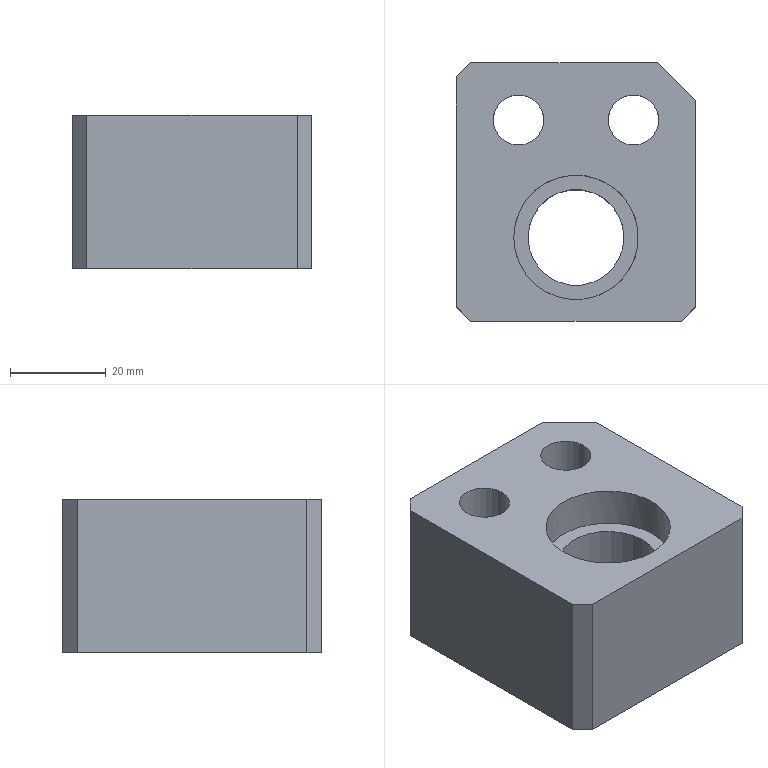Part | STEP file | lll_id3578_x_t | 1 solid | 19 faces | box 50 x 54 x 32 mm | volume 62798 mm3 | plane 13 | cylinder 6 | commonest cylinder face diameters 10.5 x2 17 x2 20 x1 26 x1
STEP:
#1=CARTESIAN_POINT('',(3209.75,-131.,77.5));
#2=VERTEX_POINT('',#1);
#3=CARTESIAN_POINT('',(3215.,-131.,77.5));
#4=DIRECTION('',(0.,0.,1.));
#5=DIRECTION('',(-1.,0.,0.));
#6=AXIS2_PLACEMENT_3D('',#3,#4,#5);
#7=CIRCLE('',#6,5.25);
#8=EDGE_CURVE('',#2,#2,#7,.T.);
#9=ORIENTED_EDGE('',*,*,#8,.T.);
#10=EDGE_LOOP('',(#9));
#11=FACE_BOUND('',#10,.T.);
#12=CARTESIAN_POINT('',(3206.5,-131.,77.5));
#13=VERTEX_POINT('',#12);
#14=CARTESIAN_POINT('',(3215.,-131.,77.5));
#15=DIRECTION('',(0.,0.,1.));
#16=DIRECTION('',(-1.,0.,0.));
#17=AXIS2_PLACEMENT_3D('',#14,#15,#16);
#18=CIRCLE('',#17,8.5);
#19=EDGE_CURVE('',#13,#13,#18,.T.);
#20=ORIENTED_EDGE('',*,*,#19,.F.);
#21=EDGE_LOOP('',(#20));
#22=FACE_BOUND('',#21,.T.);
#23=CARTESIAN_POINT('',(3215.,-131.,77.5));
#24=DIRECTION('',(0.,0.,1.));
#25=DIRECTION('',(-1.,0.,0.));
#26=AXIS2_PLACEMENT_3D('',#23,#24,#25);
#27=PLANE('',#26);
#28=ADVANCED_FACE('',(#11,#22),#27,.F.);
#29=CARTESIAN_POINT('',(3216.,-155.5,84.3));
#30=VERTEX_POINT('',#29);
#31=CARTESIAN_POINT('',(3203.,-155.5,84.3));
#32=DIRECTION('',(0.,0.,1.));
#33=DIRECTION('',(1.,0.,0.));
#34=AXIS2_PLACEMENT_3D('',#31,#32,#33);
#35=CIRCLE('',#34,13.);
#36=EDGE_CURVE('',#30,#30,#35,.T.);
#37=ORIENTED_EDGE('',*,*,#36,.T.);
#38=EDGE_LOOP('',(#37));
#39=FACE_BOUND('',#38,.T.);
#40=CARTESIAN_POINT('',(3193.,-155.5,84.3));
#41=VERTEX_POINT('',#40);
#42=CARTESIAN_POINT('',(3203.,-155.5,84.3));
#43=DIRECTION('',(0.,0.,1.));
#44=DIRECTION('',(-1.,0.,0.));
#45=AXIS2_PLACEMENT_3D('',#42,#43,#44);
#46=CIRCLE('',#45,10.);
#47=EDGE_CURVE('',#41,#41,#46,.T.);
#48=ORIENTED_EDGE('',*,*,#47,.F.);
#49=EDGE_LOOP('',(#48));
#50=FACE_BOUND('',#49,.T.);
#51=CARTESIAN_POINT('',(3203.,-146.75,84.3));
#52=DIRECTION('',(0.,0.,-1.));
#53=DIRECTION('',(0.,1.,0.));
#54=AXIS2_PLACEMENT_3D('',#51,#52,#53);
#55=PLANE('',#54);
#56=ADVANCED_FACE('',(#39,#50),#55,.F.);
#57=ORIENTED_EDGE('',*,*,#19,.T.);
#58=EDGE_LOOP('',(#57));
#59=FACE_BOUND('',#58,.T.);
#60=CARTESIAN_POINT('',(3206.5,-131.,60.5));
#61=VERTEX_POINT('',#60);
#62=CARTESIAN_POINT('',(3215.,-131.,60.5));
#63=DIRECTION('',(0.,0.,-1.));
#64=DIRECTION('',(-1.,0.,0.));
#65=AXIS2_PLACEMENT_3D('',#62,#63,#64);
#66=CIRCLE('',#65,8.5);
#67=EDGE_CURVE('',#61,#61,#66,.T.);
#68=ORIENTED_EDGE('',*,*,#67,.T.);
#69=EDGE_LOOP('',(#68));
#70=FACE_BOUND('',#69,.T.);
#71=CARTESIAN_POINT('',(3215.,-131.,60.5));
#72=DIRECTION('',(0.,0.,1.));
#73=DIRECTION('',(-1.,0.,0.));
#74=AXIS2_PLACEMENT_3D('',#71,#72,#73);
#75=CYLINDRICAL_SURFACE('',#74,8.5);
#76=ADVANCED_FACE('',(#59,#70),#75,.F.);
#77=CARTESIAN_POINT('',(3228.,-127.,60.5));
#78=VERTEX_POINT('',#77);
#79=CARTESIAN_POINT('',(3220.,-119.,60.5));
#80=VERTEX_POINT('',#79);
#81=CARTESIAN_POINT('',(3220.,-119.,60.5));
#82=DIRECTION('',(-0.7071,0.7071,0.));
#83=VECTOR('',#82,1.);
#84=LINE('',#81,#83);
#85=EDGE_CURVE('',#78,#80,#84,.T.);
#86=ORIENTED_EDGE('',*,*,#85,.T.);
#87=CARTESIAN_POINT('',(3220.,-119.,92.5));
#88=VERTEX_POINT('',#87);
#89=CARTESIAN_POINT('',(3220.,-119.,-8.5));
#90=DIRECTION('',(0.,0.,1.));
#91=VECTOR('',#90,1.);
#92=LINE('',#89,#91);
#93=EDGE_CURVE('',#80,#88,#92,.T.);
#94=ORIENTED_EDGE('',*,*,#93,.T.);
#95=CARTESIAN_POINT('',(3228.,-127.,92.5));
#96=VERTEX_POINT('',#95);
#97=CARTESIAN_POINT('',(3220.,-119.,92.5));
#98=DIRECTION('',(0.7071,-0.7071,0.));
#99=VECTOR('',#98,1.);
#100=LINE('',#97,#99);
#101=EDGE_CURVE('',#88,#96,#100,.T.);
#102=ORIENTED_EDGE('',*,*,#101,.T.);
#103=CARTESIAN_POINT('',(3228.,-127.,-8.5));
#104=DIRECTION('',(0.,0.,-1.));
#105=VECTOR('',#104,1.);
#106=LINE('',#103,#105);
#107=EDGE_CURVE('',#96,#78,#106,.T.);
#108=ORIENTED_EDGE('',*,*,#107,.T.);
#109=EDGE_LOOP('',(#86,#94,#102,#108));
#110=FACE_OUTER_BOUND('',#109,.T.);
#111=CARTESIAN_POINT('',(3220.,-119.,-8.5));
#112=DIRECTION('',(-0.7071,-0.7071,0.));
#113=DIRECTION('',(0.7071,-0.7071,0.));
#114=AXIS2_PLACEMENT_3D('',#111,#112,#113);
#115=PLANE('',#114);
#116=ADVANCED_FACE('',(#110),#115,.F.);
#117=CARTESIAN_POINT('',(3228.,-170.,92.5));
#118=VERTEX_POINT('',#117);
#119=CARTESIAN_POINT('',(3228.,-124.275,92.5));
#120=DIRECTION('',(0.,1.,0.));
#121=VECTOR('',#120,1.);
#122=LINE('',#119,#121);
#123=EDGE_CURVE('',#118,#96,#122,.T.);
#124=ORIENTED_EDGE('',*,*,#123,.F.);
#125=CARTESIAN_POINT('',(3228.,-170.,60.5));
#126=VERTEX_POINT('',#125);
#127=CARTESIAN_POINT('',(3228.,-170.,-8.5));
#128=DIRECTION('',(0.,0.,1.));
#129=VECTOR('',#128,1.);
#130=LINE('',#127,#129);
#131=EDGE_CURVE('',#126,#118,#130,.T.);
#132=ORIENTED_EDGE('',*,*,#131,.F.);
#133=CARTESIAN_POINT('',(3228.,-124.275,60.5));
#134=DIRECTION('',(0.,-1.,0.));
#135=VECTOR('',#134,1.);
#136=LINE('',#133,#135);
#137=EDGE_CURVE('',#78,#126,#136,.T.);
#138=ORIENTED_EDGE('',*,*,#137,.F.);
#139=ORIENTED_EDGE('',*,*,#107,.F.);
#140=EDGE_LOOP('',(#124,#132,#138,#139));
#141=FACE_OUTER_BOUND('',#140,.T.);
#142=CARTESIAN_POINT('',(3228.,-155.5,-8.5));
#143=DIRECTION('',(1.,0.,0.));
#144=DIRECTION('',(0.,0.,1.));
#145=AXIS2_PLACEMENT_3D('',#142,#143,#144);
#146=PLANE('',#145);
#147=ADVANCED_FACE('',(#141),#146,.T.);
#148=CARTESIAN_POINT('',(3225.,-173.,92.5));
#149=VERTEX_POINT('',#148);
#150=CARTESIAN_POINT('',(3225.,-173.,92.5));
#151=DIRECTION('',(-0.7071,-0.7071,0.));
#152=VECTOR('',#151,1.);
#153=LINE('',#150,#152);
#154=EDGE_CURVE('',#118,#149,#153,.T.);
#155=ORIENTED_EDGE('',*,*,#154,.T.);
#156=CARTESIAN_POINT('',(3225.,-173.,60.5));
#157=VERTEX_POINT('',#156);
#158=CARTESIAN_POINT('',(3225.,-173.,-8.5));
#159=DIRECTION('',(0.,0.,-1.));
#160=VECTOR('',#159,1.);
#161=LINE('',#158,#160);
#162=EDGE_CURVE('',#149,#157,#161,.T.);
#163=ORIENTED_EDGE('',*,*,#162,.T.);
#164=CARTESIAN_POINT('',(3225.,-173.,60.5));
#165=DIRECTION('',(0.7071,0.7071,0.));
#166=VECTOR('',#165,1.);
#167=LINE('',#164,#166);
#168=EDGE_CURVE('',#157,#126,#167,.T.);
#169=ORIENTED_EDGE('',*,*,#168,.T.);
#170=ORIENTED_EDGE('',*,*,#131,.T.);
#171=EDGE_LOOP('',(#155,#163,#169,#170));
#172=FACE_OUTER_BOUND('',#171,.T.);
#173=CARTESIAN_POINT('',(3225.,-173.,-8.5));
#174=DIRECTION('',(-0.7071,0.7071,0.));
#175=DIRECTION('',(-0.7071,-0.7071,0.));
#176=AXIS2_PLACEMENT_3D('',#173,#174,#175);
#177=PLANE('',#176);
#178=ADVANCED_FACE('',(#172),#177,.F.);
#179=CARTESIAN_POINT('',(3181.,-173.,92.5));
#180=VERTEX_POINT('',#179);
#181=CARTESIAN_POINT('',(3203.,-173.,92.5));
#182=DIRECTION('',(1.,0.,0.));
#183=VECTOR('',#182,1.);
#184=LINE('',#181,#183);
#185=EDGE_CURVE('',#180,#149,#184,.T.);
#186=ORIENTED_EDGE('',*,*,#185,.F.);
#187=CARTESIAN_POINT('',(3181.,-173.,60.5));
#188=VERTEX_POINT('',#187);
#189=CARTESIAN_POINT('',(3181.,-173.,-8.5));
#190=DIRECTION('',(0.,0.,1.));
#191=VECTOR('',#190,1.);
#192=LINE('',#189,#191);
#193=EDGE_CURVE('',#188,#180,#192,.T.);
#194=ORIENTED_EDGE('',*,*,#193,.F.);
#195=CARTESIAN_POINT('',(3203.,-173.,60.5));
#196=DIRECTION('',(-1.,0.,0.));
#197=VECTOR('',#196,1.);
#198=LINE('',#195,#197);
#199=EDGE_CURVE('',#157,#188,#198,.T.);
#200=ORIENTED_EDGE('',*,*,#199,.F.);
#201=ORIENTED_EDGE('',*,*,#162,.F.);
#202=EDGE_LOOP('',(#186,#194,#200,#201));
#203=FACE_OUTER_BOUND('',#202,.T.);
#204=CARTESIAN_POINT('',(3203.,-173.,-8.5));
#205=DIRECTION('',(0.,-1.,0.));
#206=DIRECTION('',(0.,0.,-1.));
#207=AXIS2_PLACEMENT_3D('',#204,#205,#206);
#208=PLANE('',#207);
#209=ADVANCED_FACE('',(#203),#208,.T.);
#210=CARTESIAN_POINT('',(3178.,-170.,92.5));
#211=VERTEX_POINT('',#210);
#212=CARTESIAN_POINT('',(3178.,-170.,92.5));
#213=DIRECTION('',(-0.7071,0.7071,0.));
#214=VECTOR('',#213,1.);
#215=LINE('',#212,#214);
#216=EDGE_CURVE('',#180,#211,#215,.T.);
#217=ORIENTED_EDGE('',*,*,#216,.T.);
#218=CARTESIAN_POINT('',(3178.,-170.,60.5));
#219=VERTEX_POINT('',#218);
#220=CARTESIAN_POINT('',(3178.,-170.,-8.5));
#221=DIRECTION('',(0.,0.,-1.));
#222=VECTOR('',#221,1.);
#223=LINE('',#220,#222);
#224=EDGE_CURVE('',#211,#219,#223,.T.);
#225=ORIENTED_EDGE('',*,*,#224,.T.);
#226=CARTESIAN_POINT('',(3178.,-170.,60.5));
#227=DIRECTION('',(0.7071,-0.7071,0.));
#228=VECTOR('',#227,1.);
#229=LINE('',#226,#228);
#230=EDGE_CURVE('',#219,#188,#229,.T.);
#231=ORIENTED_EDGE('',*,*,#230,.T.);
#232=ORIENTED_EDGE('',*,*,#193,.T.);
#233=EDGE_LOOP('',(#217,#225,#231,#232));
#234=FACE_OUTER_BOUND('',#233,.T.);
#235=CARTESIAN_POINT('',(3178.,-170.,-8.5));
#236=DIRECTION('',(0.7071,0.7071,0.));
#237=DIRECTION('',(-0.7071,0.7071,0.));
#238=AXIS2_PLACEMENT_3D('',#235,#236,#237);
#239=PLANE('',#238);
#240=ADVANCED_FACE('',(#234),#239,.F.);
#241=CARTESIAN_POINT('',(3178.,-122.,60.5));
#242=VERTEX_POINT('',#241);
#243=CARTESIAN_POINT('',(3178.,-124.275,60.5));
#244=DIRECTION('',(0.,1.,0.));
#245=VECTOR('',#244,1.);
#246=LINE('',#243,#245);
#247=EDGE_CURVE('',#219,#242,#246,.T.);
#248=ORIENTED_EDGE('',*,*,#247,.F.);
#249=ORIENTED_EDGE('',*,*,#224,.F.);
#250=CARTESIAN_POINT('',(3178.,-122.,92.5));
#251=VERTEX_POINT('',#250);
#252=CARTESIAN_POINT('',(3178.,-124.275,92.5));
#253=DIRECTION('',(0.,-1.,0.));
#254=VECTOR('',#253,1.);
#255=LINE('',#252,#254);
#256=EDGE_CURVE('',#251,#211,#255,.T.);
#257=ORIENTED_EDGE('',*,*,#256,.F.);
#258=CARTESIAN_POINT('',(3178.,-122.,-8.5));
#259=DIRECTION('',(0.,0.,1.));
#260=VECTOR('',#259,1.);
#261=LINE('',#258,#260);
#262=EDGE_CURVE('',#242,#251,#261,.T.);
#263=ORIENTED_EDGE('',*,*,#262,.F.);
#264=EDGE_LOOP('',(#248,#249,#257,#263));
#265=FACE_OUTER_BOUND('',#264,.T.);
#266=CARTESIAN_POINT('',(3178.,-155.5,-8.5));
#267=DIRECTION('',(-1.,0.,0.));
#268=DIRECTION('',(0.,0.,-1.));
#269=AXIS2_PLACEMENT_3D('',#266,#267,#268);
#270=PLANE('',#269);
#271=ADVANCED_FACE('',(#265),#270,.T.);
#272=CARTESIAN_POINT('',(3181.,-119.,92.5));
#273=VERTEX_POINT('',#272);
#274=CARTESIAN_POINT('',(3181.,-119.,92.5));
#275=DIRECTION('',(0.7071,0.7071,0.));
#276=VECTOR('',#275,1.);
#277=LINE('',#274,#276);
#278=EDGE_CURVE('',#251,#273,#277,.T.);
#279=ORIENTED_EDGE('',*,*,#278,.T.);
#280=CARTESIAN_POINT('',(3181.,-119.,60.5));
#281=VERTEX_POINT('',#280);
#282=CARTESIAN_POINT('',(3181.,-119.,-8.5));
#283=DIRECTION('',(0.,0.,-1.));
#284=VECTOR('',#283,1.);
#285=LINE('',#282,#284);
#286=EDGE_CURVE('',#273,#281,#285,.T.);
#287=ORIENTED_EDGE('',*,*,#286,.T.);
#288=CARTESIAN_POINT('',(3181.,-119.,60.5));
#289=DIRECTION('',(-0.7071,-0.7071,0.));
#290=VECTOR('',#289,1.);
#291=LINE('',#288,#290);
#292=EDGE_CURVE('',#281,#242,#291,.T.);
#293=ORIENTED_EDGE('',*,*,#292,.T.);
#294=ORIENTED_EDGE('',*,*,#262,.T.);
#295=EDGE_LOOP('',(#279,#287,#293,#294));
#296=FACE_OUTER_BOUND('',#295,.T.);
#297=CARTESIAN_POINT('',(3181.,-119.,-8.5));
#298=DIRECTION('',(0.7071,-0.7071,0.));
#299=DIRECTION('',(0.7071,0.7071,0.));
#300=AXIS2_PLACEMENT_3D('',#297,#298,#299);
#301=PLANE('',#300);
#302=ADVANCED_FACE('',(#296),#301,.F.);
#303=CARTESIAN_POINT('',(3203.,-119.,60.5));
#304=DIRECTION('',(1.,0.,0.));
#305=VECTOR('',#304,1.);
#306=LINE('',#303,#305);
#307=EDGE_CURVE('',#281,#80,#306,.T.);
#308=ORIENTED_EDGE('',*,*,#307,.F.);
#309=ORIENTED_EDGE('',*,*,#286,.F.);
#310=CARTESIAN_POINT('',(3203.,-119.,92.5));
#311=DIRECTION('',(-1.,0.,0.));
#312=VECTOR('',#311,1.);
#313=LINE('',#310,#312);
#314=EDGE_CURVE('',#88,#273,#313,.T.);
#315=ORIENTED_EDGE('',*,*,#314,.F.);
#316=ORIENTED_EDGE('',*,*,#93,.F.);
#317=EDGE_LOOP('',(#308,#309,#315,#316));
#318=FACE_OUTER_BOUND('',#317,.T.);
#319=CARTESIAN_POINT('',(3203.,-119.,-8.5));
#320=DIRECTION('',(0.,1.,0.));
#321=DIRECTION('',(0.,0.,1.));
#322=AXIS2_PLACEMENT_3D('',#319,#320,#321);
#323=PLANE('',#322);
#324=ADVANCED_FACE('',(#318),#323,.T.);
#325=CARTESIAN_POINT('',(3209.75,-131.,92.5));
#326=VERTEX_POINT('',#325);
#327=CARTESIAN_POINT('',(3215.,-131.,92.5));
#328=DIRECTION('',(0.,0.,-1.));
#329=DIRECTION('',(-1.,0.,0.));
#330=AXIS2_PLACEMENT_3D('',#327,#328,#329);
#331=CIRCLE('',#330,5.25);
#332=EDGE_CURVE('',#326,#326,#331,.T.);
#333=ORIENTED_EDGE('',*,*,#332,.F.);
#334=EDGE_LOOP('',(#333));
#335=FACE_BOUND('',#334,.T.);
#336=ORIENTED_EDGE('',*,*,#8,.F.);
#337=EDGE_LOOP('',(#336));
#338=FACE_BOUND('',#337,.T.);
#339=CARTESIAN_POINT('',(3215.,-131.,160.5));
#340=DIRECTION('',(0.,0.,1.));
#341=DIRECTION('',(-1.,0.,0.));
#342=AXIS2_PLACEMENT_3D('',#339,#340,#341);
#343=CYLINDRICAL_SURFACE('',#342,5.25);
#344=ADVANCED_FACE('',(#335,#338),#343,.F.);
#345=CARTESIAN_POINT('',(3190.,-155.5,92.5));
#346=VERTEX_POINT('',#345);
#347=CARTESIAN_POINT('',(3203.,-155.5,92.5));
#348=DIRECTION('',(0.,0.,-1.));
#349=DIRECTION('',(-1.,0.,0.));
#350=AXIS2_PLACEMENT_3D('',#347,#348,#349);
#351=CIRCLE('',#350,13.);
#352=EDGE_CURVE('',#346,#346,#351,.T.);
#353=ORIENTED_EDGE('',*,*,#352,.F.);
#354=EDGE_LOOP('',(#353));
#355=FACE_BOUND('',#354,.T.);
#356=ORIENTED_EDGE('',*,*,#36,.F.);
#357=EDGE_LOOP('',(#356));
#358=FACE_BOUND('',#357,.T.);
#359=CARTESIAN_POINT('',(3203.,-155.5,90.));
#360=DIRECTION('',(0.,0.,-1.));
#361=DIRECTION('',(0.,-1.,0.));
#362=AXIS2_PLACEMENT_3D('',#359,#360,#361);
#363=CYLINDRICAL_SURFACE('',#362,13.);
#364=ADVANCED_FACE('',(#355,#358),#363,.F.);
#365=CARTESIAN_POINT('',(3196.25,-131.,92.5));
#366=VERTEX_POINT('',#365);
#367=CARTESIAN_POINT('',(3191.,-131.,92.5));
#368=DIRECTION('',(0.,0.,1.));
#369=DIRECTION('',(1.,0.,0.));
#370=AXIS2_PLACEMENT_3D('',#367,#368,#369);
#371=CIRCLE('',#370,5.25);
#372=EDGE_CURVE('',#366,#366,#371,.T.);
#373=ORIENTED_EDGE('',*,*,#372,.F.);
#374=EDGE_LOOP('',(#373));
#375=FACE_BOUND('',#374,.T.);
#376=ORIENTED_EDGE('',*,*,#352,.T.);
#377=EDGE_LOOP('',(#376));
#378=FACE_BOUND('',#377,.T.);
#379=ORIENTED_EDGE('',*,*,#332,.T.);
#380=EDGE_LOOP('',(#379));
#381=FACE_BOUND('',#380,.T.);
#382=ORIENTED_EDGE('',*,*,#314,.T.);
#383=ORIENTED_EDGE('',*,*,#278,.F.);
#384=ORIENTED_EDGE('',*,*,#256,.T.);
#385=ORIENTED_EDGE('',*,*,#216,.F.);
#386=ORIENTED_EDGE('',*,*,#185,.T.);
#387=ORIENTED_EDGE('',*,*,#154,.F.);
#388=ORIENTED_EDGE('',*,*,#123,.T.);
#389=ORIENTED_EDGE('',*,*,#101,.F.);
#390=EDGE_LOOP('',(#382,#383,#384,#385,#386,#387,#388,#389));
#391=FACE_BOUND('',#390,.T.);
#392=CARTESIAN_POINT('',(3134.86,-124.275,92.5));
#393=DIRECTION('',(0.,0.,1.));
#394=DIRECTION('',(-1.,0.,0.));
#395=AXIS2_PLACEMENT_3D('',#392,#393,#394);
#396=PLANE('',#395);
#397=ADVANCED_FACE('',(#375,#378,#381,#391),#396,.T.);
#398=CARTESIAN_POINT('',(3213.,-155.5,60.5));
#399=VERTEX_POINT('',#398);
#400=CARTESIAN_POINT('',(3203.,-155.5,60.5));
#401=DIRECTION('',(0.,0.,1.));
#402=DIRECTION('',(1.,0.,0.));
#403=AXIS2_PLACEMENT_3D('',#400,#401,#402);
#404=CIRCLE('',#403,10.);
#405=EDGE_CURVE('',#399,#399,#404,.T.);
#406=ORIENTED_EDGE('',*,*,#405,.F.);
#407=EDGE_LOOP('',(#406));
#408=FACE_BOUND('',#407,.T.);
#409=ORIENTED_EDGE('',*,*,#47,.T.);
#410=EDGE_LOOP('',(#409));
#411=FACE_BOUND('',#410,.T.);
#412=CARTESIAN_POINT('',(3203.,-155.5,44.8));
#413=DIRECTION('',(0.,0.,-1.));
#414=DIRECTION('',(0.,-1.,0.));
#415=AXIS2_PLACEMENT_3D('',#412,#413,#414);
#416=CYLINDRICAL_SURFACE('',#415,10.);
#417=ADVANCED_FACE('',(#408,#411),#416,.F.);
#418=CARTESIAN_POINT('',(3199.5,-131.,60.5));
#419=VERTEX_POINT('',#418);
#420=CARTESIAN_POINT('',(3191.,-131.,60.5));
#421=DIRECTION('',(0.,0.,-1.));
#422=DIRECTION('',(1.,0.,0.));
#423=AXIS2_PLACEMENT_3D('',#420,#421,#422);
#424=CIRCLE('',#423,8.5);
#425=EDGE_CURVE('',#419,#419,#424,.T.);
#426=ORIENTED_EDGE('',*,*,#425,.F.);
#427=EDGE_LOOP('',(#426));
#428=FACE_BOUND('',#427,.T.);
#429=ORIENTED_EDGE('',*,*,#405,.T.);
#430=EDGE_LOOP('',(#429));
#431=FACE_BOUND('',#430,.T.);
#432=ORIENTED_EDGE('',*,*,#137,.T.);
#433=ORIENTED_EDGE('',*,*,#168,.F.);
#434=ORIENTED_EDGE('',*,*,#199,.T.);
#435=ORIENTED_EDGE('',*,*,#230,.F.);
#436=ORIENTED_EDGE('',*,*,#247,.T.);
#437=ORIENTED_EDGE('',*,*,#292,.F.);
#438=ORIENTED_EDGE('',*,*,#307,.T.);
#439=ORIENTED_EDGE('',*,*,#85,.F.);
#440=EDGE_LOOP('',(#432,#433,#434,#435,#436,#437,#438,#439));
#441=FACE_BOUND('',#440,.T.);
#442=ORIENTED_EDGE('',*,*,#67,.F.);
#443=EDGE_LOOP('',(#442));
#444=FACE_BOUND('',#443,.T.);
#445=CARTESIAN_POINT('',(3134.86,-124.275,60.5));
#446=DIRECTION('',(0.,0.,1.));
#447=DIRECTION('',(-1.,0.,0.));
#448=AXIS2_PLACEMENT_3D('',#445,#446,#447);
#449=PLANE('',#448);
#450=ADVANCED_FACE('',(#428,#431,#441,#444),#449,.F.);
#451=CARTESIAN_POINT('',(3196.25,-131.,77.5));
#452=VERTEX_POINT('',#451);
#453=CARTESIAN_POINT('',(3191.,-131.,77.5));
#454=DIRECTION('',(0.,0.,1.));
#455=DIRECTION('',(1.,0.,0.));
#456=AXIS2_PLACEMENT_3D('',#453,#454,#455);
#457=CIRCLE('',#456,5.25);
#458=EDGE_CURVE('',#452,#452,#457,.T.);
#459=ORIENTED_EDGE('',*,*,#458,.T.);
#460=EDGE_LOOP('',(#459));
#461=FACE_BOUND('',#460,.T.);
#462=CARTESIAN_POINT('',(3199.5,-131.,77.5));
#463=VERTEX_POINT('',#462);
#464=CARTESIAN_POINT('',(3191.,-131.,77.5));
#465=DIRECTION('',(0.,0.,1.));
#466=DIRECTION('',(1.,0.,0.));
#467=AXIS2_PLACEMENT_3D('',#464,#465,#466);
#468=CIRCLE('',#467,8.5);
#469=EDGE_CURVE('',#463,#463,#468,.T.);
#470=ORIENTED_EDGE('',*,*,#469,.F.);
#471=EDGE_LOOP('',(#470));
#472=FACE_BOUND('',#471,.T.);
#473=CARTESIAN_POINT('',(3191.,-131.,77.5));
#474=DIRECTION('',(0.,0.,1.));
#475=DIRECTION('',(1.,0.,0.));
#476=AXIS2_PLACEMENT_3D('',#473,#474,#475);
#477=PLANE('',#476);
#478=ADVANCED_FACE('',(#461,#472),#477,.F.);
#479=ORIENTED_EDGE('',*,*,#372,.T.);
#480=EDGE_LOOP('',(#479));
#481=FACE_BOUND('',#480,.T.);
#482=ORIENTED_EDGE('',*,*,#458,.F.);
#483=EDGE_LOOP('',(#482));
#484=FACE_BOUND('',#483,.T.);
#485=CARTESIAN_POINT('',(3191.,-131.,160.5));
#486=DIRECTION('',(0.,0.,1.));
#487=DIRECTION('',(1.,0.,0.));
#488=AXIS2_PLACEMENT_3D('',#485,#486,#487);
#489=CYLINDRICAL_SURFACE('',#488,5.25);
#490=ADVANCED_FACE('',(#481,#484),#489,.F.);
#491=ORIENTED_EDGE('',*,*,#469,.T.);
#492=EDGE_LOOP('',(#491));
#493=FACE_BOUND('',#492,.T.);
#494=ORIENTED_EDGE('',*,*,#425,.T.);
#495=EDGE_LOOP('',(#494));
#496=FACE_BOUND('',#495,.T.);
#497=CARTESIAN_POINT('',(3191.,-131.,60.5));
#498=DIRECTION('',(0.,0.,1.));
#499=DIRECTION('',(1.,0.,0.));
#500=AXIS2_PLACEMENT_3D('',#497,#498,#499);
#501=CYLINDRICAL_SURFACE('',#500,8.5);
#502=ADVANCED_FACE('',(#493,#496),#501,.F.);
#503=CLOSED_SHELL('',(#28,#56,#76,#116,#147,#178,#209,#240,#271,#302,#324,#344,#364,#397,#417,#450,#478,#490,#502));
#504=MANIFOLD_SOLID_BREP('',#503);
#505=(LENGTH_UNIT()NAMED_UNIT(*)SI_UNIT(.MILLI.,.METRE.));
#506=UNCERTAINTY_MEASURE_WITH_UNIT(LENGTH_MEASURE(0.00002),#505,'','');
#507=(NAMED_UNIT(*)PLANE_ANGLE_UNIT()SI_UNIT($,.RADIAN.));
#508=PLANE_ANGLE_MEASURE_WITH_UNIT(PLANE_ANGLE_MEASURE(0.01745),#507);
#509=DIMENSIONAL_EXPONENTS(0.,0.,0.,0.,0.,0.,0.);
#510=(CONVERSION_BASED_UNIT('DEGREE',#508)NAMED_UNIT(#509)PLANE_ANGLE_UNIT());
#511=(NAMED_UNIT(*)SI_UNIT($,.STERADIAN.)SOLID_ANGLE_UNIT());
#512=(GEOMETRIC_REPRESENTATION_CONTEXT(3)GLOBAL_UNCERTAINTY_ASSIGNED_CONTEXT((#506))GLOBAL_UNIT_ASSIGNED_CONTEXT((#505,#510,#511))REPRESENTATION_CONTEXT('',''));
#513=ADVANCED_BREP_SHAPE_REPRESENTATION('',(#504),#512);